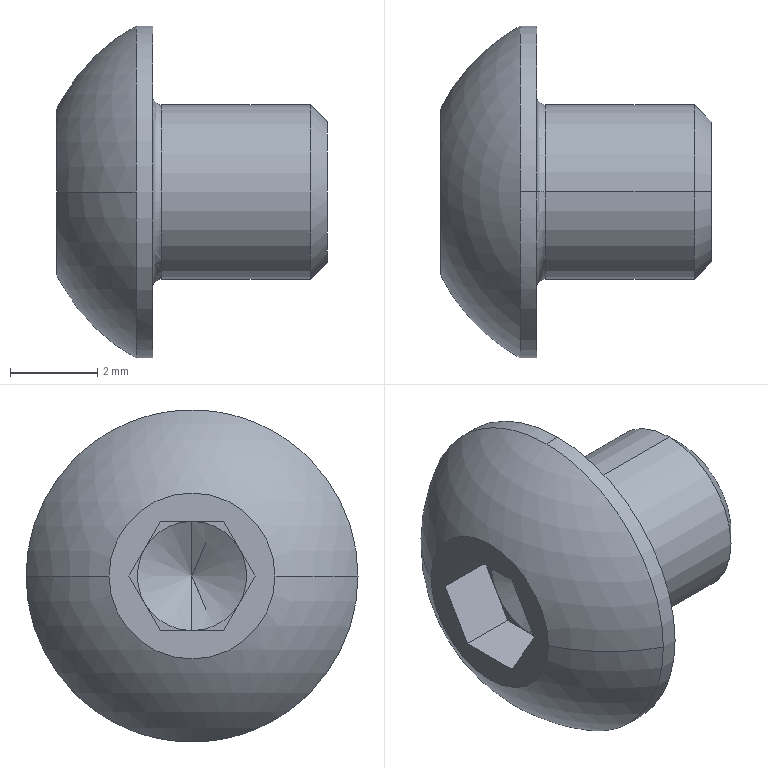Part | SolidWorks | features RevCut 2, Cut 1, Fillet 1, LPattern 1, Revolution 1 | 1 solid | 27 faces | box 6.2 x 7.6 x 7.6 mm | volume 113.262 mm3 | plane 15 | cone 4 | cylinder 4 | torus 2 | sphere 2 | commonest cylinder face diameters 4 x2 7.6 x2
STEP:
#1=CARTESIAN_POINT('',(2.022,0.,0.));
#2=VERTEX_POINT('',#1);
#3=CARTESIAN_POINT('',(1.3,0.,1.25));
#4=VERTEX_POINT('',#3);
#5=CARTESIAN_POINT('',(2.022,0.,0.));
#6=DIRECTION('',(-0.5,0.,0.866));
#7=VECTOR('',#6,1000.);
#8=LINE('',#5,#7);
#9=EDGE_CURVE('',#2,#4,#8,.T.);
#10=ORIENTED_EDGE('',*,*,#9,.F.);
#11=CARTESIAN_POINT('',(1.3,0.,-1.25));
#12=VERTEX_POINT('',#11);
#13=CARTESIAN_POINT('',(2.022,0.,0.));
#14=DIRECTION('',(-0.5,0.,-0.866));
#15=VECTOR('',#14,1000.);
#16=LINE('',#13,#15);
#17=EDGE_CURVE('',#2,#12,#16,.T.);
#18=ORIENTED_EDGE('',*,*,#17,.T.);
#19=CARTESIAN_POINT('',(1.3,-1.083,-0.625));
#20=VERTEX_POINT('',#19);
#21=CARTESIAN_POINT('',(1.3,0.,0.));
#22=DIRECTION('',(-1.,0.,0.));
#23=DIRECTION('',(0.,0.,1.));
#24=AXIS2_PLACEMENT_3D('',#21,#22,#23);
#25=CIRCLE('',#24,1.25);
#26=EDGE_CURVE('',#12,#20,#25,.T.);
#27=ORIENTED_EDGE('',*,*,#26,.T.);
#28=CARTESIAN_POINT('',(1.3,-1.083,0.625));
#29=VERTEX_POINT('',#28);
#30=CARTESIAN_POINT('',(1.3,0.,0.));
#31=DIRECTION('',(-1.,0.,0.));
#32=DIRECTION('',(0.,0.,1.));
#33=AXIS2_PLACEMENT_3D('',#30,#31,#32);
#34=CIRCLE('',#33,1.25);
#35=EDGE_CURVE('',#20,#29,#34,.T.);
#36=ORIENTED_EDGE('',*,*,#35,.T.);
#37=CARTESIAN_POINT('',(1.3,0.,0.));
#38=DIRECTION('',(-1.,0.,0.));
#39=DIRECTION('',(0.,0.,1.));
#40=AXIS2_PLACEMENT_3D('',#37,#38,#39);
#41=CIRCLE('',#40,1.25);
#42=EDGE_CURVE('',#29,#4,#41,.T.);
#43=ORIENTED_EDGE('',*,*,#42,.T.);
#44=EDGE_LOOP('',(#10,#18,#27,#36,#43));
#45=FACE_OUTER_BOUND('',#44,.T.);
#46=CARTESIAN_POINT('',(-997.978,0.,0.));
#47=DIRECTION('',(-1.,0.,0.));
#48=DIRECTION('',(0.,0.,1.));
#49=AXIS2_PLACEMENT_3D('',#46,#47,#48);
#50=CONICAL_SURFACE('',#49,1732.051,1.047);
#51=ADVANCED_FACE('',(#45),#50,.F.);
#52=CARTESIAN_POINT('',(2.2,0.,-2.2));
#53=VERTEX_POINT('',#52);
#54=CARTESIAN_POINT('',(2.2,0.,2.2));
#55=VERTEX_POINT('',#54);
#56=CARTESIAN_POINT('',(2.2,0.,0.));
#57=DIRECTION('',(-1.,0.,0.));
#58=DIRECTION('',(0.,0.,1.));
#59=AXIS2_PLACEMENT_3D('',#56,#57,#58);
#60=CIRCLE('',#59,2.2);
#61=EDGE_CURVE('',#53,#55,#60,.T.);
#62=ORIENTED_EDGE('',*,*,#61,.F.);
#63=CARTESIAN_POINT('',(2.4,0.,-2.));
#64=VERTEX_POINT('',#63);
#65=CARTESIAN_POINT('',(2.4,0.,-2.2));
#66=DIRECTION('',(0.,1.,0.));
#67=DIRECTION('',(0.,0.,1.));
#68=AXIS2_PLACEMENT_3D('',#65,#66,#67);
#69=CIRCLE('',#68,0.2);
#70=EDGE_CURVE('',#53,#64,#69,.T.);
#71=ORIENTED_EDGE('',*,*,#70,.T.);
#72=CARTESIAN_POINT('',(2.4,0.,2.));
#73=VERTEX_POINT('',#72);
#74=CARTESIAN_POINT('',(2.4,0.,0.));
#75=DIRECTION('',(1.,0.,0.));
#76=DIRECTION('',(0.,0.,1.));
#77=AXIS2_PLACEMENT_3D('',#74,#75,#76);
#78=CIRCLE('',#77,2.);
#79=EDGE_CURVE('',#73,#64,#78,.T.);
#80=ORIENTED_EDGE('',*,*,#79,.F.);
#81=CARTESIAN_POINT('',(2.4,0.,2.2));
#82=DIRECTION('',(0.,-1.,0.));
#83=DIRECTION('',(0.,0.,-1.));
#84=AXIS2_PLACEMENT_3D('',#81,#82,#83);
#85=CIRCLE('',#84,0.2);
#86=EDGE_CURVE('',#55,#73,#85,.T.);
#87=ORIENTED_EDGE('',*,*,#86,.F.);
#88=EDGE_LOOP('',(#62,#71,#80,#87));
#89=FACE_OUTER_BOUND('',#88,.T.);
#90=CARTESIAN_POINT('',(2.4,0.,0.));
#91=DIRECTION('',(-1.,0.,0.));
#92=DIRECTION('',(0.,0.,1.));
#93=AXIS2_PLACEMENT_3D('',#90,#91,#92);
#94=TOROIDAL_SURFACE('',#93,2.2,0.2);
#95=ADVANCED_FACE('',(#89),#94,.F.);
#96=CARTESIAN_POINT('',(6.2,0.,1.61));
#97=VERTEX_POINT('',#96);
#98=CARTESIAN_POINT('',(6.2,0.,-1.61));
#99=VERTEX_POINT('',#98);
#100=CARTESIAN_POINT('',(6.2,0.,0.));
#101=DIRECTION('',(-1.,0.,0.));
#102=DIRECTION('',(0.,0.,1.));
#103=AXIS2_PLACEMENT_3D('',#100,#101,#102);
#104=CIRCLE('',#103,1.61);
#105=EDGE_CURVE('',#97,#99,#104,.T.);
#106=ORIENTED_EDGE('',*,*,#105,.T.);
#107=CARTESIAN_POINT('',(5.81,0.,-2.));
#108=VERTEX_POINT('',#107);
#109=CARTESIAN_POINT('',(6.2,0.,-1.61));
#110=DIRECTION('',(-0.7071,0.,-0.7071));
#111=VECTOR('',#110,1000.);
#112=LINE('',#109,#111);
#113=EDGE_CURVE('',#99,#108,#112,.T.);
#114=ORIENTED_EDGE('',*,*,#113,.T.);
#115=CARTESIAN_POINT('',(5.81,0.,2.));
#116=VERTEX_POINT('',#115);
#117=CARTESIAN_POINT('',(5.81,0.,0.));
#118=DIRECTION('',(-1.,0.,0.));
#119=DIRECTION('',(0.,0.,1.));
#120=AXIS2_PLACEMENT_3D('',#117,#118,#119);
#121=CIRCLE('',#120,2.);
#122=EDGE_CURVE('',#116,#108,#121,.T.);
#123=ORIENTED_EDGE('',*,*,#122,.F.);
#124=CARTESIAN_POINT('',(6.2,0.,1.61));
#125=DIRECTION('',(-0.7071,0.,0.7071));
#126=VECTOR('',#125,1000.);
#127=LINE('',#124,#126);
#128=EDGE_CURVE('',#97,#116,#127,.T.);
#129=ORIENTED_EDGE('',*,*,#128,.F.);
#130=EDGE_LOOP('',(#106,#114,#123,#129));
#131=FACE_OUTER_BOUND('',#130,.T.);
#132=CARTESIAN_POINT('',(6.2,0.,0.));
#133=DIRECTION('',(-1.,0.,0.));
#134=DIRECTION('',(0.,0.,1.));
#135=AXIS2_PLACEMENT_3D('',#132,#133,#134);
#136=CONICAL_SURFACE('',#135,1.61,0.7854);
#137=ADVANCED_FACE('',(#131),#136,.T.);
#138=ORIENTED_EDGE('',*,*,#122,.T.);
#139=CARTESIAN_POINT('',(0.,0.,-2.));
#140=DIRECTION('',(-1.,0.,0.));
#141=VECTOR('',#140,1000.);
#142=LINE('',#139,#141);
#143=EDGE_CURVE('',#108,#64,#142,.T.);
#144=ORIENTED_EDGE('',*,*,#143,.T.);
#145=CARTESIAN_POINT('',(2.4,0.,0.));
#146=DIRECTION('',(1.,0.,0.));
#147=DIRECTION('',(0.,0.,1.));
#148=AXIS2_PLACEMENT_3D('',#145,#146,#147);
#149=CIRCLE('',#148,2.);
#150=EDGE_CURVE('',#64,#73,#149,.T.);
#151=ORIENTED_EDGE('',*,*,#150,.T.);
#152=CARTESIAN_POINT('',(0.,0.,2.));
#153=DIRECTION('',(-1.,0.,0.));
#154=VECTOR('',#153,1000.);
#155=LINE('',#152,#154);
#156=EDGE_CURVE('',#116,#73,#155,.T.);
#157=ORIENTED_EDGE('',*,*,#156,.F.);
#158=EDGE_LOOP('',(#138,#144,#151,#157));
#159=FACE_OUTER_BOUND('',#158,.T.);
#160=CARTESIAN_POINT('',(0.,0.,0.));
#161=DIRECTION('',(-1.,0.,0.));
#162=DIRECTION('',(0.,0.,1.));
#163=AXIS2_PLACEMENT_3D('',#160,#161,#162);
#164=CYLINDRICAL_SURFACE('',#163,2.);
#165=ADVANCED_FACE('',(#159),#164,.T.);
#166=CARTESIAN_POINT('',(2.2,0.,3.8));
#167=VERTEX_POINT('',#166);
#168=CARTESIAN_POINT('',(2.2,0.,-3.8));
#169=VERTEX_POINT('',#168);
#170=CARTESIAN_POINT('',(2.2,0.,0.));
#171=DIRECTION('',(-1.,0.,0.));
#172=DIRECTION('',(0.,0.,1.));
#173=AXIS2_PLACEMENT_3D('',#170,#171,#172);
#174=CIRCLE('',#173,3.8);
#175=EDGE_CURVE('',#167,#169,#174,.T.);
#176=ORIENTED_EDGE('',*,*,#175,.T.);
#177=CARTESIAN_POINT('',(1.82,0.,-3.8));
#178=VERTEX_POINT('',#177);
#179=CARTESIAN_POINT('',(0.,0.,-3.8));
#180=DIRECTION('',(-1.,0.,0.));
#181=VECTOR('',#180,1000.);
#182=LINE('',#179,#181);
#183=EDGE_CURVE('',#169,#178,#182,.T.);
#184=ORIENTED_EDGE('',*,*,#183,.T.);
#185=CARTESIAN_POINT('',(1.82,3.8,0.));
#186=VERTEX_POINT('',#185);
#187=CARTESIAN_POINT('',(1.82,0.,0.));
#188=DIRECTION('',(-1.,0.,0.));
#189=DIRECTION('',(0.,0.,1.));
#190=AXIS2_PLACEMENT_3D('',#187,#188,#189);
#191=CIRCLE('',#190,3.8);
#192=EDGE_CURVE('',#186,#178,#191,.T.);
#193=ORIENTED_EDGE('',*,*,#192,.F.);
#194=CARTESIAN_POINT('',(1.82,0.,3.8));
#195=VERTEX_POINT('',#194);
#196=CARTESIAN_POINT('',(1.82,0.,0.));
#197=DIRECTION('',(-1.,0.,0.));
#198=DIRECTION('',(0.,0.,1.));
#199=AXIS2_PLACEMENT_3D('',#196,#197,#198);
#200=CIRCLE('',#199,3.8);
#201=EDGE_CURVE('',#195,#186,#200,.T.);
#202=ORIENTED_EDGE('',*,*,#201,.F.);
#203=CARTESIAN_POINT('',(0.,0.,3.8));
#204=DIRECTION('',(-1.,0.,0.));
#205=VECTOR('',#204,1000.);
#206=LINE('',#203,#205);
#207=EDGE_CURVE('',#167,#195,#206,.T.);
#208=ORIENTED_EDGE('',*,*,#207,.F.);
#209=EDGE_LOOP('',(#176,#184,#193,#202,#208));
#210=FACE_OUTER_BOUND('',#209,.T.);
#211=CARTESIAN_POINT('',(0.,0.,0.));
#212=DIRECTION('',(-1.,0.,0.));
#213=DIRECTION('',(0.,0.,1.));
#214=AXIS2_PLACEMENT_3D('',#211,#212,#213);
#215=CYLINDRICAL_SURFACE('',#214,3.8);
#216=ADVANCED_FACE('',(#210),#215,.T.);
#217=ORIENTED_EDGE('',*,*,#192,.T.);
#218=CARTESIAN_POINT('',(1.82,-3.8,0.));
#219=VERTEX_POINT('',#218);
#220=CARTESIAN_POINT('',(1.82,0.,0.));
#221=DIRECTION('',(-1.,0.,0.));
#222=DIRECTION('',(0.,0.,1.));
#223=AXIS2_PLACEMENT_3D('',#220,#221,#222);
#224=CIRCLE('',#223,3.8);
#225=EDGE_CURVE('',#178,#219,#224,.T.);
#226=ORIENTED_EDGE('',*,*,#225,.T.);
#227=CARTESIAN_POINT('',(0.,-1.9,0.));
#228=VERTEX_POINT('',#227);
#229=CARTESIAN_POINT('',(3.885,0.,0.));
#230=DIRECTION('',(0.,0.,-1.));
#231=DIRECTION('',(0.,1.,0.));
#232=AXIS2_PLACEMENT_3D('',#229,#230,#231);
#233=CIRCLE('',#232,4.325);
#234=EDGE_CURVE('',#219,#228,#233,.T.);
#235=ORIENTED_EDGE('',*,*,#234,.T.);
#236=CARTESIAN_POINT('',(0.,1.9,0.));
#237=VERTEX_POINT('',#236);
#238=CARTESIAN_POINT('',(0.,0.,0.));
#239=DIRECTION('',(-1.,0.,0.));
#240=DIRECTION('',(0.,0.,1.));
#241=AXIS2_PLACEMENT_3D('',#238,#239,#240);
#242=CIRCLE('',#241,1.9);
#243=EDGE_CURVE('',#237,#228,#242,.T.);
#244=ORIENTED_EDGE('',*,*,#243,.F.);
#245=CARTESIAN_POINT('',(3.885,0.,0.));
#246=DIRECTION('',(0.,0.,1.));
#247=DIRECTION('',(1.,0.,0.));
#248=AXIS2_PLACEMENT_3D('',#245,#246,#247);
#249=CIRCLE('',#248,4.325);
#250=EDGE_CURVE('',#186,#237,#249,.T.);
#251=ORIENTED_EDGE('',*,*,#250,.F.);
#252=EDGE_LOOP('',(#217,#226,#235,#244,#251));
#253=FACE_OUTER_BOUND('',#252,.T.);
#254=CARTESIAN_POINT('',(3.885,0.,0.));
#255=DIRECTION('',(0.,0.,-1.));
#256=DIRECTION('',(0.,1.,0.));
#257=AXIS2_PLACEMENT_3D('',#254,#255,#256);
#258=SPHERICAL_SURFACE('',#257,4.325);
#259=ADVANCED_FACE('',(#253),#258,.T.);
#260=ORIENTED_EDGE('',*,*,#243,.T.);
#261=CARTESIAN_POINT('',(0.,0.,0.));
#262=DIRECTION('',(-1.,0.,0.));
#263=DIRECTION('',(0.,0.,1.));
#264=AXIS2_PLACEMENT_3D('',#261,#262,#263);
#265=CIRCLE('',#264,1.9);
#266=EDGE_CURVE('',#228,#237,#265,.T.);
#267=ORIENTED_EDGE('',*,*,#266,.T.);
#268=EDGE_LOOP('',(#260,#267));
#269=FACE_OUTER_BOUND('',#268,.T.);
#270=CARTESIAN_POINT('',(0.,0.7217,1.25));
#271=VERTEX_POINT('',#270);
#272=CARTESIAN_POINT('',(0.,-0.7217,1.25));
#273=VERTEX_POINT('',#272);
#274=CARTESIAN_POINT('',(0.,-0.7217,1.25));
#275=DIRECTION('',(0.,-1.,0.));
#276=VECTOR('',#275,1000.);
#277=LINE('',#274,#276);
#278=EDGE_CURVE('',#271,#273,#277,.T.);
#279=ORIENTED_EDGE('',*,*,#278,.T.);
#280=CARTESIAN_POINT('',(0.,-1.443,0.));
#281=VERTEX_POINT('',#280);
#282=CARTESIAN_POINT('',(0.,-1.443,0.));
#283=DIRECTION('',(0.,-0.5,-0.866));
#284=VECTOR('',#283,1000.);
#285=LINE('',#282,#284);
#286=EDGE_CURVE('',#273,#281,#285,.T.);
#287=ORIENTED_EDGE('',*,*,#286,.T.);
#288=CARTESIAN_POINT('',(0.,-0.7217,-1.25));
#289=VERTEX_POINT('',#288);
#290=CARTESIAN_POINT('',(0.,-0.7217,-1.25));
#291=DIRECTION('',(0.,0.5,-0.866));
#292=VECTOR('',#291,1000.);
#293=LINE('',#290,#292);
#294=EDGE_CURVE('',#281,#289,#293,.T.);
#295=ORIENTED_EDGE('',*,*,#294,.T.);
#296=CARTESIAN_POINT('',(0.,0.7217,-1.25));
#297=VERTEX_POINT('',#296);
#298=CARTESIAN_POINT('',(0.,0.7217,-1.25));
#299=DIRECTION('',(0.,1.,0.));
#300=VECTOR('',#299,1000.);
#301=LINE('',#298,#300);
#302=EDGE_CURVE('',#289,#297,#301,.T.);
#303=ORIENTED_EDGE('',*,*,#302,.T.);
#304=CARTESIAN_POINT('',(0.,1.443,0.));
#305=VERTEX_POINT('',#304);
#306=CARTESIAN_POINT('',(0.,1.443,0.));
#307=DIRECTION('',(0.,0.5,0.866));
#308=VECTOR('',#307,1000.);
#309=LINE('',#306,#308);
#310=EDGE_CURVE('',#297,#305,#309,.T.);
#311=ORIENTED_EDGE('',*,*,#310,.T.);
#312=CARTESIAN_POINT('',(0.,0.7217,1.25));
#313=DIRECTION('',(0.,-0.5,0.866));
#314=VECTOR('',#313,1000.);
#315=LINE('',#312,#314);
#316=EDGE_CURVE('',#305,#271,#315,.T.);
#317=ORIENTED_EDGE('',*,*,#316,.T.);
#318=EDGE_LOOP('',(#279,#287,#295,#303,#311,#317));
#319=FACE_BOUND('',#318,.T.);
#320=CARTESIAN_POINT('',(0.,0.,0.));
#321=DIRECTION('',(-1.,0.,0.));
#322=DIRECTION('',(0.,0.,1.));
#323=AXIS2_PLACEMENT_3D('',#320,#321,#322);
#324=PLANE('',#323);
#325=ADVANCED_FACE('',(#269,#319),#324,.T.);
#326=ORIENTED_EDGE('',*,*,#234,.F.);
#327=CARTESIAN_POINT('',(1.82,0.,0.));
#328=DIRECTION('',(-1.,0.,0.));
#329=DIRECTION('',(0.,0.,1.));
#330=AXIS2_PLACEMENT_3D('',#327,#328,#329);
#331=CIRCLE('',#330,3.8);
#332=EDGE_CURVE('',#219,#195,#331,.T.);
#333=ORIENTED_EDGE('',*,*,#332,.T.);
#334=ORIENTED_EDGE('',*,*,#201,.T.);
#335=ORIENTED_EDGE('',*,*,#250,.T.);
#336=ORIENTED_EDGE('',*,*,#266,.F.);
#337=EDGE_LOOP('',(#326,#333,#334,#335,#336));
#338=FACE_OUTER_BOUND('',#337,.T.);
#339=CARTESIAN_POINT('',(3.885,0.,0.));
#340=DIRECTION('',(0.,0.,-1.));
#341=DIRECTION('',(0.,1.,0.));
#342=AXIS2_PLACEMENT_3D('',#339,#340,#341);
#343=SPHERICAL_SURFACE('',#342,4.325);
#344=ADVANCED_FACE('',(#338),#343,.T.);
#345=ORIENTED_EDGE('',*,*,#183,.F.);
#346=CARTESIAN_POINT('',(2.2,0.,0.));
#347=DIRECTION('',(-1.,0.,0.));
#348=DIRECTION('',(0.,0.,1.));
#349=AXIS2_PLACEMENT_3D('',#346,#347,#348);
#350=CIRCLE('',#349,3.8);
#351=EDGE_CURVE('',#169,#167,#350,.T.);
#352=ORIENTED_EDGE('',*,*,#351,.T.);
#353=ORIENTED_EDGE('',*,*,#207,.T.);
#354=ORIENTED_EDGE('',*,*,#332,.F.);
#355=ORIENTED_EDGE('',*,*,#225,.F.);
#356=EDGE_LOOP('',(#345,#352,#353,#354,#355));
#357=FACE_OUTER_BOUND('',#356,.T.);
#358=CARTESIAN_POINT('',(0.,0.,0.));
#359=DIRECTION('',(-1.,0.,0.));
#360=DIRECTION('',(0.,0.,1.));
#361=AXIS2_PLACEMENT_3D('',#358,#359,#360);
#362=CYLINDRICAL_SURFACE('',#361,3.8);
#363=ADVANCED_FACE('',(#357),#362,.T.);
#364=CARTESIAN_POINT('',(2.2,0.,0.));
#365=DIRECTION('',(-1.,0.,0.));
#366=DIRECTION('',(0.,0.,1.));
#367=AXIS2_PLACEMENT_3D('',#364,#365,#366);
#368=CIRCLE('',#367,2.2);
#369=EDGE_CURVE('',#55,#53,#368,.T.);
#370=ORIENTED_EDGE('',*,*,#369,.T.);
#371=ORIENTED_EDGE('',*,*,#61,.T.);
#372=EDGE_LOOP('',(#370,#371));
#373=FACE_BOUND('',#372,.T.);
#374=ORIENTED_EDGE('',*,*,#175,.F.);
#375=ORIENTED_EDGE('',*,*,#351,.F.);
#376=EDGE_LOOP('',(#374,#375));
#377=FACE_OUTER_BOUND('',#376,.T.);
#378=CARTESIAN_POINT('',(2.2,2.,0.));
#379=DIRECTION('',(-1.,0.,0.));
#380=DIRECTION('',(0.,0.,1.));
#381=AXIS2_PLACEMENT_3D('',#378,#379,#380);
#382=PLANE('',#381);
#383=ADVANCED_FACE('',(#373,#377),#382,.F.);
#384=ORIENTED_EDGE('',*,*,#143,.F.);
#385=CARTESIAN_POINT('',(5.81,0.,0.));
#386=DIRECTION('',(-1.,0.,0.));
#387=DIRECTION('',(0.,0.,1.));
#388=AXIS2_PLACEMENT_3D('',#385,#386,#387);
#389=CIRCLE('',#388,2.);
#390=EDGE_CURVE('',#108,#116,#389,.T.);
#391=ORIENTED_EDGE('',*,*,#390,.T.);
#392=ORIENTED_EDGE('',*,*,#156,.T.);
#393=ORIENTED_EDGE('',*,*,#79,.T.);
#394=EDGE_LOOP('',(#384,#391,#392,#393));
#395=FACE_OUTER_BOUND('',#394,.T.);
#396=CARTESIAN_POINT('',(0.,0.,0.));
#397=DIRECTION('',(-1.,0.,0.));
#398=DIRECTION('',(0.,0.,1.));
#399=AXIS2_PLACEMENT_3D('',#396,#397,#398);
#400=CYLINDRICAL_SURFACE('',#399,2.);
#401=ADVANCED_FACE('',(#395),#400,.T.);
#402=ORIENTED_EDGE('',*,*,#113,.F.);
#403=CARTESIAN_POINT('',(6.2,0.,0.));
#404=DIRECTION('',(-1.,0.,0.));
#405=DIRECTION('',(0.,0.,1.));
#406=AXIS2_PLACEMENT_3D('',#403,#404,#405);
#407=CIRCLE('',#406,1.61);
#408=EDGE_CURVE('',#99,#97,#407,.T.);
#409=ORIENTED_EDGE('',*,*,#408,.T.);
#410=ORIENTED_EDGE('',*,*,#128,.T.);
#411=ORIENTED_EDGE('',*,*,#390,.F.);
#412=EDGE_LOOP('',(#402,#409,#410,#411));
#413=FACE_OUTER_BOUND('',#412,.T.);
#414=CARTESIAN_POINT('',(6.2,0.,0.));
#415=DIRECTION('',(-1.,0.,0.));
#416=DIRECTION('',(0.,0.,1.));
#417=AXIS2_PLACEMENT_3D('',#414,#415,#416);
#418=CONICAL_SURFACE('',#417,1.61,0.7854);
#419=ADVANCED_FACE('',(#413),#418,.T.);
#420=ORIENTED_EDGE('',*,*,#105,.F.);
#421=ORIENTED_EDGE('',*,*,#408,.F.);
#422=EDGE_LOOP('',(#420,#421));
#423=FACE_OUTER_BOUND('',#422,.T.);
#424=CARTESIAN_POINT('',(6.2,0.,0.));
#425=DIRECTION('',(-1.,0.,0.));
#426=DIRECTION('',(0.,0.,1.));
#427=AXIS2_PLACEMENT_3D('',#424,#425,#426);
#428=PLANE('',#427);
#429=ADVANCED_FACE('',(#423),#428,.F.);
#430=ORIENTED_EDGE('',*,*,#70,.F.);
#431=ORIENTED_EDGE('',*,*,#369,.F.);
#432=ORIENTED_EDGE('',*,*,#86,.T.);
#433=ORIENTED_EDGE('',*,*,#150,.F.);
#434=EDGE_LOOP('',(#430,#431,#432,#433));
#435=FACE_OUTER_BOUND('',#434,.T.);
#436=CARTESIAN_POINT('',(2.4,0.,0.));
#437=DIRECTION('',(-1.,0.,0.));
#438=DIRECTION('',(0.,0.,1.));
#439=AXIS2_PLACEMENT_3D('',#436,#437,#438);
#440=TOROIDAL_SURFACE('',#439,2.2,0.2);
#441=ADVANCED_FACE('',(#435),#440,.F.);
#442=CARTESIAN_POINT('',(1.3,-0.7217,1.25));
#443=VERTEX_POINT('',#442);
#444=CARTESIAN_POINT('',(1.3,-1.443,0.));
#445=DIRECTION('',(0.,-0.5,-0.866));
#446=VECTOR('',#445,1000.);
#447=LINE('',#444,#446);
#448=EDGE_CURVE('',#443,#29,#447,.T.);
#449=ORIENTED_EDGE('',*,*,#448,.T.);
#450=CARTESIAN_POINT('',(1.3,-1.443,0.));
#451=VERTEX_POINT('',#450);
#452=CARTESIAN_POINT('',(1.3,-1.443,0.));
#453=DIRECTION('',(0.,-0.5,-0.866));
#454=VECTOR('',#453,1000.);
#455=LINE('',#452,#454);
#456=EDGE_CURVE('',#29,#451,#455,.T.);
#457=ORIENTED_EDGE('',*,*,#456,.T.);
#458=CARTESIAN_POINT('',(1.3,-1.443,0.));
#459=DIRECTION('',(-1.,0.,0.));
#460=VECTOR('',#459,1000.);
#461=LINE('',#458,#460);
#462=EDGE_CURVE('',#451,#281,#461,.T.);
#463=ORIENTED_EDGE('',*,*,#462,.T.);
#464=ORIENTED_EDGE('',*,*,#286,.F.);
#465=CARTESIAN_POINT('',(1.3,-0.7217,1.25));
#466=DIRECTION('',(-1.,0.,0.));
#467=VECTOR('',#466,1000.);
#468=LINE('',#465,#467);
#469=EDGE_CURVE('',#443,#273,#468,.T.);
#470=ORIENTED_EDGE('',*,*,#469,.F.);
#471=EDGE_LOOP('',(#449,#457,#463,#464,#470));
#472=FACE_OUTER_BOUND('',#471,.T.);
#473=CARTESIAN_POINT('',(1.3,-1.443,0.));
#474=DIRECTION('',(0.,0.866,-0.5));
#475=DIRECTION('',(0.,0.5,0.866));
#476=AXIS2_PLACEMENT_3D('',#473,#474,#475);
#477=PLANE('',#476);
#478=ADVANCED_FACE('',(#472),#477,.T.);
#479=CARTESIAN_POINT('',(1.3,-0.7217,-1.25));
#480=DIRECTION('',(0.,0.5,-0.866));
#481=VECTOR('',#480,1000.);
#482=LINE('',#479,#481);
#483=EDGE_CURVE('',#451,#20,#482,.T.);
#484=ORIENTED_EDGE('',*,*,#483,.T.);
#485=CARTESIAN_POINT('',(1.3,-0.7217,-1.25));
#486=VERTEX_POINT('',#485);
#487=CARTESIAN_POINT('',(1.3,-0.7217,-1.25));
#488=DIRECTION('',(0.,0.5,-0.866));
#489=VECTOR('',#488,1000.);
#490=LINE('',#487,#489);
#491=EDGE_CURVE('',#20,#486,#490,.T.);
#492=ORIENTED_EDGE('',*,*,#491,.T.);
#493=CARTESIAN_POINT('',(1.3,-0.7217,-1.25));
#494=DIRECTION('',(-1.,0.,0.));
#495=VECTOR('',#494,1000.);
#496=LINE('',#493,#495);
#497=EDGE_CURVE('',#486,#289,#496,.T.);
#498=ORIENTED_EDGE('',*,*,#497,.T.);
#499=ORIENTED_EDGE('',*,*,#294,.F.);
#500=ORIENTED_EDGE('',*,*,#462,.F.);
#501=EDGE_LOOP('',(#484,#492,#498,#499,#500));
#502=FACE_OUTER_BOUND('',#501,.T.);
#503=CARTESIAN_POINT('',(1.3,-0.7217,-1.25));
#504=DIRECTION('',(0.,0.866,0.5));
#505=DIRECTION('',(0.,-0.5,0.866));
#506=AXIS2_PLACEMENT_3D('',#503,#504,#505);
#507=PLANE('',#506);
#508=ADVANCED_FACE('',(#502),#507,.T.);
#509=CARTESIAN_POINT('',(1.3,0.7217,-1.25));
#510=DIRECTION('',(0.,1.,0.));
#511=VECTOR('',#510,1000.);
#512=LINE('',#509,#511);
#513=EDGE_CURVE('',#486,#12,#512,.T.);
#514=ORIENTED_EDGE('',*,*,#513,.T.);
#515=CARTESIAN_POINT('',(1.3,0.7217,-1.25));
#516=VERTEX_POINT('',#515);
#517=CARTESIAN_POINT('',(1.3,0.7217,-1.25));
#518=DIRECTION('',(0.,1.,0.));
#519=VECTOR('',#518,1000.);
#520=LINE('',#517,#519);
#521=EDGE_CURVE('',#12,#516,#520,.T.);
#522=ORIENTED_EDGE('',*,*,#521,.T.);
#523=CARTESIAN_POINT('',(1.3,0.7217,-1.25));
#524=DIRECTION('',(-1.,0.,0.));
#525=VECTOR('',#524,1000.);
#526=LINE('',#523,#525);
#527=EDGE_CURVE('',#516,#297,#526,.T.);
#528=ORIENTED_EDGE('',*,*,#527,.T.);
#529=ORIENTED_EDGE('',*,*,#302,.F.);
#530=ORIENTED_EDGE('',*,*,#497,.F.);
#531=EDGE_LOOP('',(#514,#522,#528,#529,#530));
#532=FACE_OUTER_BOUND('',#531,.T.);
#533=CARTESIAN_POINT('',(1.3,0.7217,-1.25));
#534=DIRECTION('',(0.,0.,1.));
#535=DIRECTION('',(0.,-1.,0.));
#536=AXIS2_PLACEMENT_3D('',#533,#534,#535);
#537=PLANE('',#536);
#538=ADVANCED_FACE('',(#532),#537,.T.);
#539=CARTESIAN_POINT('',(1.3,1.083,-0.625));
#540=VERTEX_POINT('',#539);
#541=CARTESIAN_POINT('',(1.3,1.443,0.));
#542=DIRECTION('',(0.,0.5,0.866));
#543=VECTOR('',#542,1000.);
#544=LINE('',#541,#543);
#545=EDGE_CURVE('',#516,#540,#544,.T.);
#546=ORIENTED_EDGE('',*,*,#545,.T.);
#547=CARTESIAN_POINT('',(1.3,1.443,0.));
#548=VERTEX_POINT('',#547);
#549=CARTESIAN_POINT('',(1.3,1.443,0.));
#550=DIRECTION('',(0.,0.5,0.866));
#551=VECTOR('',#550,1000.);
#552=LINE('',#549,#551);
#553=EDGE_CURVE('',#540,#548,#552,.T.);
#554=ORIENTED_EDGE('',*,*,#553,.T.);
#555=CARTESIAN_POINT('',(1.3,1.443,0.));
#556=DIRECTION('',(-1.,0.,0.));
#557=VECTOR('',#556,1000.);
#558=LINE('',#555,#557);
#559=EDGE_CURVE('',#548,#305,#558,.T.);
#560=ORIENTED_EDGE('',*,*,#559,.T.);
#561=ORIENTED_EDGE('',*,*,#310,.F.);
#562=ORIENTED_EDGE('',*,*,#527,.F.);
#563=EDGE_LOOP('',(#546,#554,#560,#561,#562));
#564=FACE_OUTER_BOUND('',#563,.T.);
#565=CARTESIAN_POINT('',(1.3,1.443,0.));
#566=DIRECTION('',(0.,-0.866,0.5));
#567=DIRECTION('',(0.,-0.5,-0.866));
#568=AXIS2_PLACEMENT_3D('',#565,#566,#567);
#569=PLANE('',#568);
#570=ADVANCED_FACE('',(#564),#569,.T.);
#571=CARTESIAN_POINT('',(1.3,1.083,0.625));
#572=VERTEX_POINT('',#571);
#573=CARTESIAN_POINT('',(1.3,0.7217,1.25));
#574=DIRECTION('',(0.,-0.5,0.866));
#575=VECTOR('',#574,1000.);
#576=LINE('',#573,#575);
#577=EDGE_CURVE('',#548,#572,#576,.T.);
#578=ORIENTED_EDGE('',*,*,#577,.T.);
#579=CARTESIAN_POINT('',(1.3,0.7217,1.25));
#580=VERTEX_POINT('',#579);
#581=CARTESIAN_POINT('',(1.3,0.7217,1.25));
#582=DIRECTION('',(0.,-0.5,0.866));
#583=VECTOR('',#582,1000.);
#584=LINE('',#581,#583);
#585=EDGE_CURVE('',#572,#580,#584,.T.);
#586=ORIENTED_EDGE('',*,*,#585,.T.);
#587=CARTESIAN_POINT('',(1.3,0.7217,1.25));
#588=DIRECTION('',(-1.,0.,0.));
#589=VECTOR('',#588,1000.);
#590=LINE('',#587,#589);
#591=EDGE_CURVE('',#580,#271,#590,.T.);
#592=ORIENTED_EDGE('',*,*,#591,.T.);
#593=ORIENTED_EDGE('',*,*,#316,.F.);
#594=ORIENTED_EDGE('',*,*,#559,.F.);
#595=EDGE_LOOP('',(#578,#586,#592,#593,#594));
#596=FACE_OUTER_BOUND('',#595,.T.);
#597=CARTESIAN_POINT('',(1.3,0.7217,1.25));
#598=DIRECTION('',(0.,-0.866,-0.5));
#599=DIRECTION('',(0.,0.5,-0.866));
#600=AXIS2_PLACEMENT_3D('',#597,#598,#599);
#601=PLANE('',#600);
#602=ADVANCED_FACE('',(#596),#601,.T.);
#603=CARTESIAN_POINT('',(1.3,-0.7217,1.25));
#604=DIRECTION('',(0.,-1.,0.));
#605=VECTOR('',#604,1000.);
#606=LINE('',#603,#605);
#607=EDGE_CURVE('',#580,#4,#606,.T.);
#608=ORIENTED_EDGE('',*,*,#607,.T.);
#609=CARTESIAN_POINT('',(1.3,-0.7217,1.25));
#610=DIRECTION('',(0.,-1.,0.));
#611=VECTOR('',#610,1000.);
#612=LINE('',#609,#611);
#613=EDGE_CURVE('',#4,#443,#612,.T.);
#614=ORIENTED_EDGE('',*,*,#613,.T.);
#615=ORIENTED_EDGE('',*,*,#469,.T.);
#616=ORIENTED_EDGE('',*,*,#278,.F.);
#617=ORIENTED_EDGE('',*,*,#591,.F.);
#618=EDGE_LOOP('',(#608,#614,#615,#616,#617));
#619=FACE_OUTER_BOUND('',#618,.T.);
#620=CARTESIAN_POINT('',(1.3,-0.7217,1.25));
#621=DIRECTION('',(0.,0.,-1.));
#622=DIRECTION('',(0.,1.,0.));
#623=AXIS2_PLACEMENT_3D('',#620,#621,#622);
#624=PLANE('',#623);
#625=ADVANCED_FACE('',(#619),#624,.T.);
#626=CARTESIAN_POINT('',(1.3,0.,0.));
#627=DIRECTION('',(-1.,0.,0.));
#628=DIRECTION('',(0.,0.,1.));
#629=AXIS2_PLACEMENT_3D('',#626,#627,#628);
#630=CIRCLE('',#629,1.25);
#631=EDGE_CURVE('',#540,#12,#630,.T.);
#632=ORIENTED_EDGE('',*,*,#631,.F.);
#633=ORIENTED_EDGE('',*,*,#545,.F.);
#634=ORIENTED_EDGE('',*,*,#521,.F.);
#635=EDGE_LOOP('',(#632,#633,#634));
#636=FACE_OUTER_BOUND('',#635,.T.);
#637=CARTESIAN_POINT('',(1.3,-2.165,-1.25));
#638=DIRECTION('',(1.,0.,0.));
#639=DIRECTION('',(0.,0.,-1.));
#640=AXIS2_PLACEMENT_3D('',#637,#638,#639);
#641=PLANE('',#640);
#642=ADVANCED_FACE('',(#636),#641,.F.);
#643=CARTESIAN_POINT('',(1.3,0.,0.));
#644=DIRECTION('',(-1.,0.,0.));
#645=DIRECTION('',(0.,0.,1.));
#646=AXIS2_PLACEMENT_3D('',#643,#644,#645);
#647=CIRCLE('',#646,1.25);
#648=EDGE_CURVE('',#572,#540,#647,.T.);
#649=ORIENTED_EDGE('',*,*,#648,.F.);
#650=ORIENTED_EDGE('',*,*,#577,.F.);
#651=ORIENTED_EDGE('',*,*,#553,.F.);
#652=EDGE_LOOP('',(#649,#650,#651));
#653=FACE_OUTER_BOUND('',#652,.T.);
#654=CARTESIAN_POINT('',(1.3,-2.165,-1.25));
#655=DIRECTION('',(1.,0.,0.));
#656=DIRECTION('',(0.,0.,-1.));
#657=AXIS2_PLACEMENT_3D('',#654,#655,#656);
#658=PLANE('',#657);
#659=ADVANCED_FACE('',(#653),#658,.F.);
#660=CARTESIAN_POINT('',(1.3,0.,0.));
#661=DIRECTION('',(-1.,0.,0.));
#662=DIRECTION('',(0.,0.,1.));
#663=AXIS2_PLACEMENT_3D('',#660,#661,#662);
#664=CIRCLE('',#663,1.25);
#665=EDGE_CURVE('',#4,#572,#664,.T.);
#666=ORIENTED_EDGE('',*,*,#665,.F.);
#667=ORIENTED_EDGE('',*,*,#607,.F.);
#668=ORIENTED_EDGE('',*,*,#585,.F.);
#669=EDGE_LOOP('',(#666,#667,#668));
#670=FACE_OUTER_BOUND('',#669,.T.);
#671=CARTESIAN_POINT('',(1.3,-2.165,-1.25));
#672=DIRECTION('',(1.,0.,0.));
#673=DIRECTION('',(0.,0.,-1.));
#674=AXIS2_PLACEMENT_3D('',#671,#672,#673);
#675=PLANE('',#674);
#676=ADVANCED_FACE('',(#670),#675,.F.);
#677=ORIENTED_EDGE('',*,*,#42,.F.);
#678=ORIENTED_EDGE('',*,*,#448,.F.);
#679=ORIENTED_EDGE('',*,*,#613,.F.);
#680=EDGE_LOOP('',(#677,#678,#679));
#681=FACE_OUTER_BOUND('',#680,.T.);
#682=CARTESIAN_POINT('',(1.3,-2.165,-1.25));
#683=DIRECTION('',(1.,0.,0.));
#684=DIRECTION('',(0.,0.,-1.));
#685=AXIS2_PLACEMENT_3D('',#682,#683,#684);
#686=PLANE('',#685);
#687=ADVANCED_FACE('',(#681),#686,.F.);
#688=ORIENTED_EDGE('',*,*,#35,.F.);
#689=ORIENTED_EDGE('',*,*,#483,.F.);
#690=ORIENTED_EDGE('',*,*,#456,.F.);
#691=EDGE_LOOP('',(#688,#689,#690));
#692=FACE_OUTER_BOUND('',#691,.T.);
#693=CARTESIAN_POINT('',(1.3,-2.165,-1.25));
#694=DIRECTION('',(1.,0.,0.));
#695=DIRECTION('',(0.,0.,-1.));
#696=AXIS2_PLACEMENT_3D('',#693,#694,#695);
#697=PLANE('',#696);
#698=ADVANCED_FACE('',(#692),#697,.F.);
#699=ORIENTED_EDGE('',*,*,#26,.F.);
#700=ORIENTED_EDGE('',*,*,#513,.F.);
#701=ORIENTED_EDGE('',*,*,#491,.F.);
#702=EDGE_LOOP('',(#699,#700,#701));
#703=FACE_OUTER_BOUND('',#702,.T.);
#704=CARTESIAN_POINT('',(1.3,-2.165,-1.25));
#705=DIRECTION('',(1.,0.,0.));
#706=DIRECTION('',(0.,0.,-1.));
#707=AXIS2_PLACEMENT_3D('',#704,#705,#706);
#708=PLANE('',#707);
#709=ADVANCED_FACE('',(#703),#708,.F.);
#710=ORIENTED_EDGE('',*,*,#17,.F.);
#711=ORIENTED_EDGE('',*,*,#9,.T.);
#712=ORIENTED_EDGE('',*,*,#665,.T.);
#713=ORIENTED_EDGE('',*,*,#648,.T.);
#714=ORIENTED_EDGE('',*,*,#631,.T.);
#715=EDGE_LOOP('',(#710,#711,#712,#713,#714));
#716=FACE_OUTER_BOUND('',#715,.T.);
#717=CARTESIAN_POINT('',(-997.978,0.,0.));
#718=DIRECTION('',(-1.,0.,0.));
#719=DIRECTION('',(0.,0.,1.));
#720=AXIS2_PLACEMENT_3D('',#717,#718,#719);
#721=CONICAL_SURFACE('',#720,1732.051,1.047);
#722=ADVANCED_FACE('',(#716),#721,.F.);
#723=CLOSED_SHELL('',(#51,#95,#137,#165,#216,#259,#325,#344,#363,#383,#401,#419,#429,#441,#478,#508,#538,#570,#602,#625,#642,#659,#676,#687,#698,#709,#722));
#724=MANIFOLD_SOLID_BREP('',#723);
#725=CARTESIAN_POINT('',(0.,0.,0.));
#726=DIRECTION('',(0.,0.,1.));
#727=DIRECTION('',(1.,0.,0.));
#728=AXIS2_PLACEMENT_3D('',#725,#726,#727);
#729=(LENGTH_UNIT()NAMED_UNIT(*)SI_UNIT(.MILLI.,.METRE.));
#730=UNCERTAINTY_MEASURE_WITH_UNIT(LENGTH_MEASURE(0.00001),#729,'','');
#731=(NAMED_UNIT(*)PLANE_ANGLE_UNIT()SI_UNIT($,.RADIAN.));
#732=(NAMED_UNIT(*)SI_UNIT($,.STERADIAN.)SOLID_ANGLE_UNIT());
#733=(GEOMETRIC_REPRESENTATION_CONTEXT(3)GLOBAL_UNCERTAINTY_ASSIGNED_CONTEXT((#730))GLOBAL_UNIT_ASSIGNED_CONTEXT((#729,#731,#732))REPRESENTATION_CONTEXT('',''));
#734=ADVANCED_BREP_SHAPE_REPRESENTATION('',(#724,#728),#733);